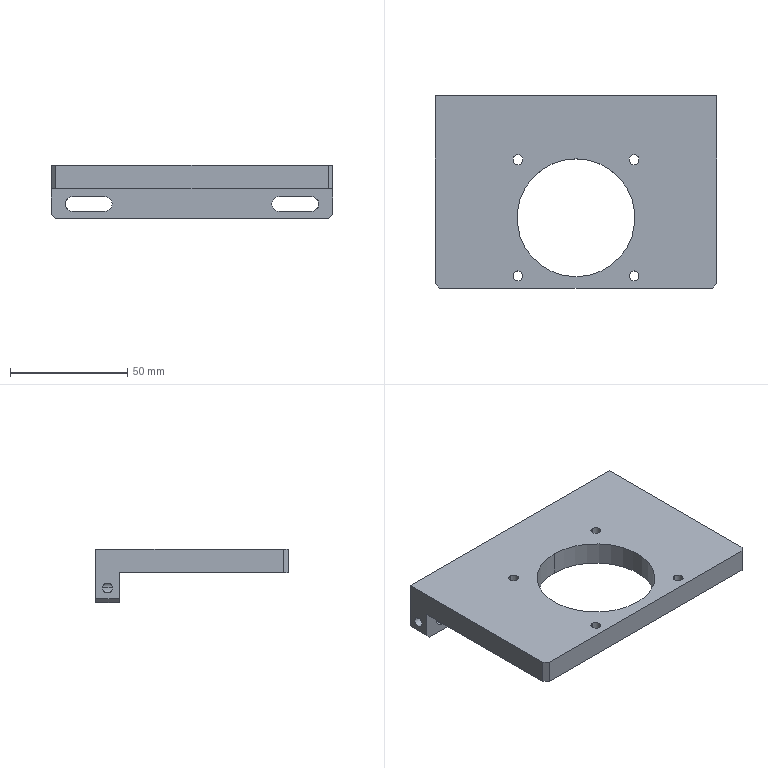NC program | NX | posted with a generic post | part box 120 x 82 x 22.8 mm
Whole program:
N10 G17 G21 G94 G90
(FLOOR_WALL_COPY , TOOL : D80)
N12 T19 M6
N14 G54
N16 G17 G0 G90 X-103. Y40.997 B0. C0. S6500 M3
N18 G43 Z30. H19
N20 Z9.
N22 G94 G1 Z6. F1500.
N24 X-100.
N26 X100.
N28 Y15.999
N30 X-100.
N32 Y-9.
N34 X100.
N36 X103.
N38 Z9.
N40 G0 Z30.
N42 X-103. Y40.997
N44 Z8.
N46 G1 Z5.
N48 X-100.
N50 X100.
N52 Y15.999
N54 X-100.
N56 Y-9.
N58 X100.
N60 X103.
N62 Z8.
N64 G0 Z30.
N66 X-103. Y40.997
N68 Z7.
N70 G1 Z4.
N72 X-100.
N74 X100.
N76 Y15.999
N78 X-100.
N80 Y-9.
N82 X100.
N84 X103.
N86 Z7.
N88 G0 Z30.
N90 X-103. Y40.997
N92 Z6.
N94 G1 Z3.
N96 X-100.
N98 X100.
N100 Y15.999
N102 X-100.
N104 Y-9.
N106 X100.
N108 X103.
N110 Z6.
N112 G0 Z30.
N114 X-103. Y40.997
N116 Z5.
N118 G1 Z2.
N120 X-100.
N122 X100.
N124 Y15.999
N126 X-100.
N128 Y-9.
N130 X100.
N132 X103.
N134 Z5.
N136 G0 Z30.
N138 X-103. Y40.997
N140 Z4.
N142 G1 Z1.
N144 X-100.
N146 X100.
N148 Y15.999
N150 X-100.
N152 Y-9.
N154 X100.
N156 X103.
N158 Z4.
N160 G0 Z30.
N162 X-103. Y40.997
N164 Z3.
N166 G1 Z0.
N168 X-100.
N170 X100.
N172 Y15.999
N174 X-100.
N176 Y-9.
N178 X100.
N180 X103.
N182 Z3.
N184 G0 Z30.
N186 M5
(FLOOR_WALL_1 , TOOL : D10)
N188 T15 M6
N190 G54
N192 G17 G0 G90 X4.33 Y-47.5 B0. C0. S9500 M3
N194 G43 Z30. H15
N196 Z0.208
N198 G94 G1 Z-0.792 F3000.
N200 X0.866 Y-41.5
N202 G3 X0. Y-41. R1.
N204 G1 X-58.
N206 X-60. Y-39.
N208 Y25.9
N210 X60.
N212 Y-39.
N214 X58. Y-41.
N216 X0.
N218 Y-34.
N220 X-53.
N222 Y18.9
N224 X53.
N226 Y-34.
N228 X0.
N230 Y-27.
N232 X-46.
N234 Y11.9
N236 X46.
N238 Y-27.
N240 X0.
N242 Y-20.
N244 X-39.
N246 Y4.9
N248 X39.
N250 Y-20.
N252 X0.
N254 Y-13.
N256 X-32.
N258 Y-2.1
N260 X32.
N262 Y-13.
N264 X0.
N266 Y-8.5
N268 X-27.5
N270 Y-6.6
N272 X27.5
N274 Y-8.5
N276 X0.
N278 G3 X-0.866 Y-9. R1.
N280 G1 Z0.208
N282 G0 X4.33 Y-47.5 Z-0.785
N284 G1 Z-1.785
N286 X0.866 Y-41.5
N288 G3 X0. Y-41. R1.
N290 G1 X-58.
N292 X-60. Y-39.
N294 Y25.9
N296 X60.
N298 Y-39.
N300 X58. Y-41.
N302 X0.
N304 Y-34.
N306 X-53.
N308 Y18.9
N310 X53.
N312 Y-34.
N314 X0.
N316 Y-27.
N318 X-46.
N320 Y11.9
N322 X46.
N324 Y-27.
N326 X0.
N328 Y-20.
N330 X-39.
N332 Y4.9
N334 X39.
N336 Y-20.
N338 X0.
N340 Y-13.
N342 X-32.
N344 Y-2.1
N346 X32.
N348 Y-13.
N350 X0.
N352 Y-8.5
N354 X-27.5
N356 Y-6.6
N358 X27.5
N360 Y-8.5
N362 X0.
N364 G3 X-0.866 Y-9. R1.
N366 G1 Z-0.785
N368 G0 X4.33 Y-47.5 Z-1.777
N370 G1 Z-2.777
N372 X0.866 Y-41.5
N374 G3 X0. Y-41. R1.
N376 G1 X-58.
N378 X-60. Y-39.
N380 Y25.9
N382 X60.
N384 Y-39.
N386 X58. Y-41.
N388 X0.
N390 Y-34.
N392 X-53.
N394 Y18.9
N396 X53.
N398 Y-34.
N400 X0.
N402 Y-27.
N404 X-46.
N406 Y11.9
N408 X46.
N410 Y-27.
N412 X0.
N414 Y-20.
N416 X-39.
N418 Y4.9
N420 X39.
N422 Y-20.
N424 X0.
N426 Y-13.
N428 X-32.
N430 Y-2.1
N432 X32.
N434 Y-13.
N436 X0.
N438 Y-8.5
N440 X-27.5
N442 Y-6.6
N444 X27.5
N446 Y-8.5
N448 X0.
N450 G3 X-0.866 Y-9. R1.
N452 G1 Z-1.777
N454 G0 X4.33 Y-47.5 Z-2.769
N456 G1 Z-3.769
N458 X0.866 Y-41.5
N460 G3 X0. Y-41. R1.
N462 G1 X-58.
N464 X-60. Y-39.
N466 Y25.9
N468 X60.
N470 Y-39.
N472 X58. Y-41.
N474 X0.
N476 Y-34.
N478 X-53.
N480 Y18.9
N482 X53.
N484 Y-34.
N486 X0.
N488 Y-27.
N490 X-46.
N492 Y11.9
N494 X46.
N496 Y-27.
N498 X0.
N500 Y-20.
N502 X-39.
N504 Y4.9
N506 X39.
N508 Y-20.
N510 X0.
N512 Y-13.
N514 X-32.
N516 Y-2.1
N518 X32.
N520 Y-13.
N522 X0.
N524 Y-8.5
N526 X-27.5
N528 Y-6.6
N530 X27.5
N532 Y-8.5
N534 X0.
N536 G3 X-0.866 Y-9. R1.
N538 G1 Z-2.769
N540 G0 X4.33 Y-47.5 Z-3.762
N542 G1 Z-4.762
N544 X0.866 Y-41.5
N546 G3 X0. Y-41. R1.
N548 G1 X-58.
N550 X-60. Y-39.
N552 Y25.9
N554 X60.
N556 Y-39.
N558 X58. Y-41.
N560 X0.
N562 Y-34.
N564 X-53.
N566 Y18.9
N568 X53.
N570 Y-34.
N572 X0.
N574 Y-27.
N576 X-46.
N578 Y11.9
N580 X46.
N582 Y-27.
N584 X0.
N586 Y-20.
N588 X-39.
N590 Y4.9
N592 X39.
N594 Y-20.
N596 X0.
N598 Y-13.
N600 X-32.
N602 Y-2.1
N604 X32.
N606 Y-13.
N608 X0.
N610 Y-8.5
N612 X-27.5
N614 Y-6.6
N616 X27.5
N618 Y-8.5
N620 X0.
N622 G3 X-0.866 Y-9. R1.
N624 G1 Z-3.762
N626 G0 X4.33 Y-47.5 Z-4.754
N628 G1 Z-5.754
N630 X0.866 Y-41.5
N632 G3 X0. Y-41. R1.
N634 G1 X-58.
N636 X-60. Y-39.
N638 Y25.9
N640 X60.
N642 Y-39.
N644 X58. Y-41.
N646 X0.
N648 Y-34.
N650 X-53.
N652 Y18.9
N654 X53.
N656 Y-34.
N658 X0.
N660 Y-27.
N662 X-46.
N664 Y11.9
N666 X46.
N668 Y-27.
N670 X0.
N672 Y-20.
N674 X-39.
N676 Y4.9
N678 X39.
N680 Y-20.
N682 X0.
N684 Y-13.
N686 X-32.
N688 Y-2.1
N690 X32.
N692 Y-13.
N694 X0.
N696 Y-8.5
N698 X-27.5
N700 Y-6.6
N702 X27.5
N704 Y-8.5
N706 X0.
N708 G3 X-0.866 Y-9. R1.
N710 G1 Z-4.754
N712 G0 X4.33 Y-47.5 Z-5.746
N714 G1 Z-6.746
N716 X0.866 Y-41.5
N718 G3 X0. Y-41. R1.
N720 G1 X-58.
N722 X-60. Y-39.
N724 Y25.9
N726 X60.
N728 Y-39.
N730 X58. Y-41.
N732 X0.
N734 Y-34.
N736 X-53.
N738 Y18.9
N740 X53.
N742 Y-34.
N744 X0.
N746 Y-27.
N748 X-46.
N750 Y11.9
N752 X46.
N754 Y-27.
N756 X0.
N758 Y-20.
N760 X-39.
N762 Y4.9
N764 X39.
N766 Y-20.
N768 X0.
N770 Y-13.
N772 X-32.
N774 Y-2.1
N776 X32.
N778 Y-13.
N780 X0.
N782 Y-8.5
N784 X-27.5
N786 Y-6.6
N788 X27.5
N790 Y-8.5
N792 X0.
N794 G3 X-0.866 Y-9. R1.
N796 G1 Z-5.746
N798 G0 X4.33 Y-47.5 Z-6.738
N800 G1 Z-7.738
N802 X0.866 Y-41.5
N804 G3 X0. Y-41. R1.
N806 G1 X-58.
N808 X-60. Y-39.
N810 Y25.9
N812 X60.
N814 Y-39.
N816 X58. Y-41.
N818 X0.
N820 Y-34.
N822 X-53.
N824 Y18.9
N826 X53.
N828 Y-34.
N830 X0.
N832 Y-27.
N834 X-46.
N836 Y11.9
N838 X46.
N840 Y-27.
N842 X0.
N844 Y-20.
N846 X-39.
N848 Y4.9
N850 X39.
N852 Y-20.
N854 X0.
N856 Y-13.
N858 X-32.
N860 Y-2.1
N862 X32.
N864 Y-13.
N866 X0.
N868 Y-8.5
N870 X-27.5
N872 Y-6.6
N874 X27.5
N876 Y-8.5
N878 X0.
N880 G3 X-0.866 Y-9. R1.
N882 G1 Z-6.738
N884 G0 X4.33 Y-47.5 Z-7.731
N886 G1 Z-8.731
N888 X0.866 Y-41.5
N890 G3 X0. Y-41. R1.
N892 G1 X-58.
N894 X-60. Y-39.
N896 Y25.9
N898 X60.
N900 Y-39.
N902 X58. Y-41.
N904 X0.
N906 Y-34.
N908 X-53.
N910 Y18.9
N912 X53.
N914 Y-34.
N916 X0.
N918 Y-27.
N920 X-46.
N922 Y11.9
N924 X46.
N926 Y-27.
N928 X0.
N930 Y-20.
N932 X-39.
N934 Y4.9
N936 X39.
N938 Y-20.
N940 X0.
N942 Y-13.
N944 X-32.
N946 Y-2.1
N948 X32.
N950 Y-13.
N952 X0.
N954 Y-8.5
N956 X-27.5
N958 Y-6.6
N960 X27.5
N962 Y-8.5
N964 X0.
N966 G3 X-0.866 Y-9. R1.
N968 G1 Z-7.731
N970 G0 X4.33 Y-47.5 Z-8.723
N972 G1 Z-9.723
N974 X0.866 Y-41.5
N976 G3 X0. Y-41. R1.
N978 G1 X-58.
N980 X-60. Y-39.
N982 Y25.9
N984 X60.
N986 Y-39.
N988 X58. Y-41.
N990 X0.
N992 Y-34.
N994 X-53.
N996 Y18.9
N998 X53.
N1000 Y-34.
N1002 X0.
N1004 Y-27.
N1006 X-46.
N1008 Y11.9
N1010 X46.
N1012 Y-27.
N1014 X0.
N1016 Y-20.
N1018 X-39.
N1020 Y4.9
N1022 X39.
N1024 Y-20.
N1026 X0.
N1028 Y-13.
N1030 X-32.
N1032 Y-2.1
N1034 X32.
N1036 Y-13.
N1038 X0.
N1040 Y-8.5
N1042 X-27.5
N1044 Y-6.6
N1046 X27.5
N1048 Y-8.5
N1050 X0.
N1052 G3 X-0.866 Y-9. R1.
N1054 G1 Z-8.723
N1056 G0 X4.33 Y-47.5 Z-9.715
N1058 G1 Z-10.715
N1060 X0.866 Y-41.5
N1062 G3 X0. Y-41. R1.
N1064 G1 X-58.
N1066 X-60. Y-39.
N1068 Y25.9
N1070 X60.
N1072 Y-39.
N1074 X58. Y-41.
N1076 X0.
N1078 Y-34.
N1080 X-53.
N1082 Y18.9
N1084 X53.
N1086 Y-34.
N1088 X0.
N1090 Y-27.
N1092 X-46.
N1094 Y11.9
N1096 X46.
N1098 Y-27.
N1100 X0.
N1102 Y-20.
N1104 X-39.
N1106 Y4.9
N1108 X39.
N1110 Y-20.
N1112 X0.
N1114 Y-13.
N1116 X-32.
N1118 Y-2.1
N1120 X32.
N1122 Y-13.
N1124 X0.
N1126 Y-8.5
N1128 X-27.5
N1130 Y-6.6
N1132 X27.5
N1134 Y-8.5
N1136 X0.
N1138 G3 X-0.866 Y-9. R1.
N1140 G1 Z-9.715
N1142 G0 X4.33 Y-47.5 Z-10.708
N1144 G1 Z-11.708
N1146 X0.866 Y-41.5
N1148 G3 X0. Y-41. R1.
N1150 G1 X-58.
N1152 X-60. Y-39.
N1154 Y25.9
N1156 X60.
N1158 Y-39.
N1160 X58. Y-41.
N1162 X0.
N1164 Y-34.
N1166 X-53.
N1168 Y18.9
N1170 X53.
N1172 Y-34.
N1174 X0.
N1176 Y-27.
N1178 X-46.
N1180 Y11.9
N1182 X46.
N1184 Y-27.
N1186 X0.
N1188 Y-20.
N1190 X-39.
N1192 Y4.9
N1194 X39.
N1196 Y-20.
N1198 X0.
N1200 Y-13.
N1202 X-32.
N1204 Y-2.1
N1206 X32.
N1208 Y-13.
N1210 X0.
N1212 Y-8.5
N1214 X-27.5
N1216 Y-6.6
N1218 X27.5
N1220 Y-8.5
N1222 X0.
N1224 G3 X-0.866 Y-9. R1.
N1226 G1 Z-10.708
N1228 G0 X4.33 Y-47.5 Z-11.7
N1230 G1 Z-12.7
N1232 X0.866 Y-41.5
N1234 G3 X0. Y-41. R1.
N1236 G1 X-58.
N1238 X-60. Y-39.
N1240 Y25.9
N1242 X60.
N1244 Y-39.
N1246 X58. Y-41.
N1248 X0.
N1250 Y-34.
N1252 X-53.
N1254 Y18.9
N1256 X53.
N1258 Y-34.
N1260 X0.
N1262 Y-27.
N1264 X-46.
N1266 Y11.9
N1268 X46.
N1270 Y-27.
N1272 X0.
N1274 Y-20.
N1276 X-39.
N1278 Y4.9
N1280 X39.
N1282 Y-20.
N1284 X0.
N1286 Y-13.
N1288 X-32.
N1290 Y-2.1
N1292 X32.
N1294 Y-13.
N1296 X0.
N1298 Y-8.5
N1300 X-27.5
N1302 Y-6.6
N1304 X27.5
N1306 Y-8.5
N1308 X0.
N1310 G3 X-0.866 Y-9. R1.
N1312 G1 Z-11.7
N1314 G0 Z30.
N1316 M5
(FLOOR_WALL_1_COPY , TOOL : D10JING)
N1318 T14 M6
N1320 G54
N1322 G17 G0 G90 X66.165 Y-42.015 B0. C0. S9500 M3
N1324 G43 Z30. H14
N1326 Z-11.8
N1328 G94 G1 Z-12.8 F1500.
N1330 X65.866 Y-41.497
N1332 G3 X65. Y-40.997 R1.
N1334 G1 X-65.
N1336 Y-36.247
N1338 X65.
N1340 Y-31.497
N1342 X-65.
N1344 Y-26.748
N1346 X65.
N1348 Y-21.998
N1350 X-65.
N1352 Y-17.248
N1354 X65.
N1356 Y-12.498
N1358 X-65.
N1360 Y-7.749
N1362 X65.
N1364 Y-2.999
N1366 X-65.
N1368 Y1.751
N1370 X65.
N1372 Y6.501
N1374 X-65.
N1376 Y11.251
N1378 X65.
N1380 Y16.
N1382 X-65.
N1384 Y20.75
N1386 X65.
N1388 Y25.5
N1390 X-65.
N1392 G3 X-65.866 Y25. R1.
N1394 G1 X-66.5 Y23.902
N1396 Z-11.8
N1398 G0 X66.5 Y24.402
N1400 G1 Z-12.8
N1402 X65.866 Y25.5
N1404 G3 X65. Y26. R1.
N1406 G1 X-65.
N1408 G3 X-65.866 Y25.5 R1.
N1410 G1 X-66.5 Y24.402
N1412 Z-11.8
N1414 G0 Z30.
N1416 M5
(PLANAR_MILL_COPY , TOOL : D6A45)
N1418 T01 M6
N1420 G54
N1422 G17 G0 G90 X0.866 Y29.6 B0. C0. S9500 M3
N1424 G43 Z30. H1
N1426 Z0.5
N1428 G94 G1 Z-1. F1250.
N1430 G3 X0. Y30.1 R1.
N1432 G1 X-60.
N1434 G2 X-60.9 Y31. R0.9
N1436 G1 Y41.
N1438 G2 X-60. Y41.9 R0.9
N1440 G1 X60.
N1442 G2 X60.9 Y41. R0.9
N1444 G1 Y31.
N1446 G2 X60. Y30.1 R0.9
N1448 G1 X0.
N1450 G3 X-0.866 Y29.6 R1.
N1452 G1 Z0.5
N1454 G0 Z30.
(PLANAR_MILL_COPY_COPY_1 , TOOL : D6A45)
N1456 X-62.4 Y29.73
N1458 Z-1.
N1460 G1 Z-2.5
N1462 X-61.7 Y30.134
N1464 G3 X-61.2 Y31. R1.
N1466 G1 Y41.
N1468 G3 X-61.7 Y41.866 R1.
N1470 G1 X-62.4 Y42.27
N1472 Z-1.
N1474 G0 Z30.
N1476 Y29.441
N1478 Z-1.
N1480 G1 Z-2.5
N1482 X-61.2 Y30.134
N1484 G3 X-60.7 Y31. R1.
N1486 G1 Y41.
N1488 G3 X-61.2 Y41.866 R1.
N1490 G1 X-62.4 Y42.559
N1492 Z-1.
N1494 G0 Z30.
N1496 X62.4 Y42.27
N1498 Z-1.
N1500 G1 Z-2.5
N1502 X61.7 Y41.866
N1504 G3 X61.2 Y41. R1.
N1506 G1 Y31.
N1508 G3 X61.7 Y30.134 R1.
N1510 G1 X62.4 Y29.73
N1512 Z-1.
N1514 G0 Z30.
N1516 Y42.559
N1518 Z-1.
N1520 G1 Z-2.5
N1522 X61.2 Y41.866
N1524 G3 X60.7 Y41. R1.
N1526 G1 Y31.
N1528 G3 X61.2 Y30.134 R1.
N1530 G1 X62.4 Y29.441
N1532 Z-1.
N1534 G0 Z30.
(PLANAR_MILL_COPY_COPY , TOOL : D6A45)
N1536 X25.949 Y-35.619
N1538 Z-12.3
N1540 G1 Y-35.479 Z-12.338
N1542 X25.618 Y-34.879 Z-12.521
N1544 X25.019 Y-34.549 Z-12.704
N1546 X24.479 Z-12.849
N1548 X23.879 Y-34.879 Z-13.033
N1550 X23.549 Y-35.479 Z-13.216
N1552 Y-36.019 Z-13.361
N1554 X23.879 Y-36.618 Z-13.544
N1556 X24.479 Y-36.949 Z-13.728
N1558 X24.749 Z-13.8
N1560 G3 X25.949 Y-35.749 R1.2
N1562 X24.749 Y-36.949 R-1.2
N1564 X25.615 Y-36.449 R1.
N1566 G1 Z-12.3
N1568 G0 Z30.
N1570 X-1.291 Y-33.964
N1572 Z-12.3
N1574 G1 Z-13.8
N1576 X-0.866 Y-34.7
N1578 G3 X0. Y-35.2 R1.
N1580 X24.2 Y-11. R24.2
N1582 X0. Y-35.2 R-24.2
N1584 X0.866 Y-34.7 R1.
N1586 G1 X1.291 Y-33.964
N1588 Z-12.3
N1590 G0 Z30.
N1592 X23.549 Y13.619
N1594 Z-12.3
N1596 G1 Y13.479 Z-12.338
N1598 X23.879 Y12.879 Z-12.521
N1600 X24.479 Y12.549 Z-12.704
N1602 X25.019 Z-12.849
N1604 X25.618 Y12.879 Z-13.033
N1606 X25.949 Y13.479 Z-13.216
N1608 Y14.019 Z-13.361
N1610 X25.618 Y14.618 Z-13.544
N1612 X25.019 Y14.949 Z-13.728
N1614 X24.749 Z-13.8
N1616 G3 X23.549 Y13.749 R1.2
N1618 X24.749 Y14.949 R-1.2
N1620 X23.883 Y14.449 R1.
N1622 G1 Z-12.3
N1624 G0 Z30.
N1626 X62.501 Y27.26
N1628 Z-12.3
N1630 G1 Z-13.8
N1632 X61.893 Y27.52
N1634 G3 X60.9 Y27.4 R1.
N1636 G1 Y-38.959
N1638 G2 X60.607 Y-39.666 R1.
N1640 G1 X58.666 Y-41.607
N1642 G2 X57.959 Y-41.9 R1.
N1644 G1 X-57.959
N1646 G2 X-58.666 Y-41.607 R1.
N1648 G1 X-60.607 Y-39.666
N1650 G2 X-60.9 Y-38.959 R1.
N1652 G1 Y27.4
N1654 G3 X-61.893 Y27.52 R1.
N1656 G1 X-62.501 Y27.26
N1658 Z-12.3
N1660 G0 Z30.
N1662 X-25.949 Y13.619
N1664 Z-12.3
N1666 G1 Y13.479 Z-12.338
N1668 X-25.618 Y12.879 Z-12.521
N1670 X-25.019 Y12.549 Z-12.704
N1672 X-24.479 Z-12.849
N1674 X-23.879 Y12.879 Z-13.033
N1676 X-23.549 Y13.479 Z-13.216
N1678 Y14.019 Z-13.361
N1680 X-23.879 Y14.618 Z-13.544
N1682 X-24.479 Y14.949 Z-13.728
N1684 X-24.749 Z-13.8
N1686 G3 X-25.949 Y13.749 R1.2
N1688 X-24.749 Y14.949 R-1.2
N1690 X-25.615 Y14.449 R1.
N1692 G1 Z-12.3
N1694 G0 Z30.
N1696 X-23.549 Y-35.619
N1698 Z-12.3
N1700 G1 Y-35.479 Z-12.338
N1702 X-23.879 Y-34.879 Z-12.521
N1704 X-24.479 Y-34.549 Z-12.704
N1706 X-25.019 Z-12.849
N1708 X-25.618 Y-34.879 Z-13.033
N1710 X-25.949 Y-35.479 Z-13.216
N1712 Y-36.019 Z-13.361
N1714 X-25.618 Y-36.618 Z-13.544
N1716 X-25.019 Y-36.949 Z-13.728
N1718 X-24.749 Z-13.8
N1720 G3 X-23.549 Y-35.749 R1.2
N1722 X-24.749 Y-36.949 R-1.2
N1724 X-23.883 Y-36.449 R1.
N1726 G1 Z-12.3
N1728 G0 Z30.
N1730 M5
N1732 M2